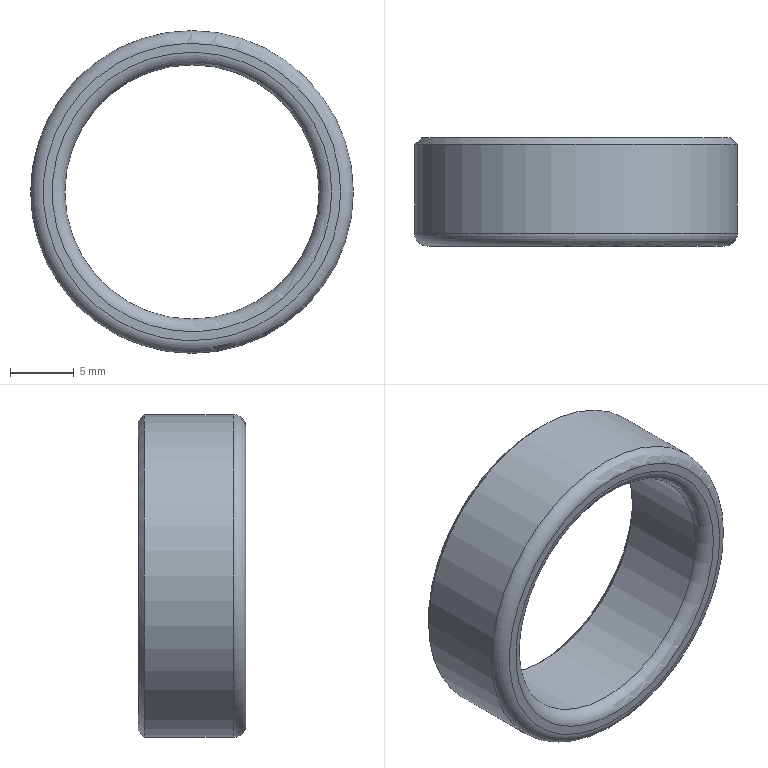Part | STEP file | BK-20_id1170_x_t | 1 solid | 8 faces | box 25.4 x 8.5 x 25.4 mm | volume 1588 mm3 | cylinder 2 | cone 2 | plane 2 | torus 2 | commonest cylinder face diameters 20 x1 25.4 x1
STEP:
#1=CARTESIAN_POINT('',(0.,0.,0.));
#2=DIRECTION('',(0.,0.,1.));
#3=DIRECTION('',(1.,0.,0.));
#4=AXIS2_PLACEMENT_3D('',#1,#2,#3);
#5=CARTESIAN_POINT('',(-258.5,510.436,-165.5));
#6=VERTEX_POINT('',#5);
#7=CARTESIAN_POINT('',(-268.5,510.436,-165.5));
#8=DIRECTION('',(0.,-1.,0.));
#9=DIRECTION('',(1.,0.,0.));
#10=AXIS2_PLACEMENT_3D('',#7,#8,#9);
#11=CIRCLE('',#10,10.);
#12=CARTESIAN_POINT('',(-268.5,494.874,-165.5));
#13=DIRECTION('',(0.,-1.,0.));
#14=DIRECTION('',(1.,0.,0.));
#15=AXIS2_PLACEMENT_3D('',#12,#13,#14);
#16=CYLINDRICAL_SURFACE('',#15,10.);
#17=CARTESIAN_POINT('',(0.,-15.562));
#18=DIRECTION('',(1.,0.));
#19=VECTOR('',#18,1.);
#20=LINE('',#17,#19);
#21=(GEOMETRIC_REPRESENTATION_CONTEXT(2)PARAMETRIC_REPRESENTATION_CONTEXT()REPRESENTATION_CONTEXT('',''));
#22=DEFINITIONAL_REPRESENTATION('',(#20),#21);
#23=PCURVE('',#16,#22);
#24=CARTESIAN_POINT('',(-268.5,510.436,-165.5));
#25=DIRECTION('',(0.,-1.,0.));
#26=DIRECTION('',(1.,0.,0.));
#27=AXIS2_PLACEMENT_3D('',#24,#25,#26);
#28=TOROIDAL_SURFACE('',#27,11.,1.);
#29=CARTESIAN_POINT('',(0.,9.425));
#30=DIRECTION('',(1.,0.));
#31=VECTOR('',#30,1.);
#32=LINE('',#29,#31);
#33=(GEOMETRIC_REPRESENTATION_CONTEXT(2)PARAMETRIC_REPRESENTATION_CONTEXT()REPRESENTATION_CONTEXT('',''));
#34=DEFINITIONAL_REPRESENTATION('',(#32),#33);
#35=PCURVE('',#28,#34);
#36=SURFACE_CURVE('',#11,(#23,#35),.PCURVE_S1.);
#37=EDGE_CURVE('',#6,#6,#36,.T.);
#38=ORIENTED_EDGE('',*,*,#37,.F.);
#39=CARTESIAN_POINT('',(-258.5,517.436,-165.5));
#40=VERTEX_POINT('',#39);
#41=CARTESIAN_POINT('',(-258.5,517.436,-165.5));
#42=CARTESIAN_POINT('',(-258.5,510.436,-165.5));
#43=B_SPLINE_CURVE_WITH_KNOTS('',1,(#41,#42),.UNSPECIFIED.,.F.,.F.,(2,2),(-22.562,-15.562),.PIECEWISE_BEZIER_KNOTS.);
#44=CARTESIAN_POINT('',(0.,0.));
#45=DIRECTION('',(0.,1.));
#46=VECTOR('',#45,1.);
#47=LINE('',#44,#46);
#48=(GEOMETRIC_REPRESENTATION_CONTEXT(2)PARAMETRIC_REPRESENTATION_CONTEXT()REPRESENTATION_CONTEXT('',''));
#49=DEFINITIONAL_REPRESENTATION('',(#47),#48);
#50=PCURVE('',#16,#49);
#51=CARTESIAN_POINT('',(6.283,0.));
#52=DIRECTION('',(0.,1.));
#53=VECTOR('',#52,1.);
#54=LINE('',#51,#53);
#55=(GEOMETRIC_REPRESENTATION_CONTEXT(2)PARAMETRIC_REPRESENTATION_CONTEXT()REPRESENTATION_CONTEXT('',''));
#56=DEFINITIONAL_REPRESENTATION('',(#54),#55);
#57=PCURVE('',#16,#56);
#58=SEAM_CURVE('',#43,(#50,#57),.PCURVE_S1.);
#59=EDGE_CURVE('',#40,#6,#58,.T.);
#60=ORIENTED_EDGE('',*,*,#59,.F.);
#61=CARTESIAN_POINT('',(-278.5,517.436,-165.5));
#62=VERTEX_POINT('',#61);
#63=CARTESIAN_POINT('',(-268.5,517.436,-165.5));
#64=DIRECTION('',(0.,1.,0.));
#65=DIRECTION('',(-1.,0.,0.));
#66=AXIS2_PLACEMENT_3D('',#63,#64,#65);
#67=CIRCLE('',#66,10.);
#68=CARTESIAN_POINT('',(3.142,-22.562));
#69=DIRECTION('',(-1.,0.));
#70=VECTOR('',#69,1.);
#71=LINE('',#68,#70);
#72=(GEOMETRIC_REPRESENTATION_CONTEXT(2)PARAMETRIC_REPRESENTATION_CONTEXT()REPRESENTATION_CONTEXT('',''));
#73=DEFINITIONAL_REPRESENTATION('',(#71),#72);
#74=PCURVE('',#16,#73);
#75=CARTESIAN_POINT('',(-268.5,517.936,-165.5));
#76=DIRECTION('',(0.,1.,0.));
#77=DIRECTION('',(-1.,0.,0.));
#78=AXIS2_PLACEMENT_3D('',#75,#76,#77);
#79=CONICAL_SURFACE('',#78,10.5,0.7854);
#80=CARTESIAN_POINT('',(0.,-0.5));
#81=DIRECTION('',(1.,0.));
#82=VECTOR('',#81,1.);
#83=LINE('',#80,#82);
#84=(GEOMETRIC_REPRESENTATION_CONTEXT(2)PARAMETRIC_REPRESENTATION_CONTEXT()REPRESENTATION_CONTEXT('',''));
#85=DEFINITIONAL_REPRESENTATION('',(#83),#84);
#86=PCURVE('',#79,#85);
#87=SURFACE_CURVE('',#67,(#74,#86),.PCURVE_S1.);
#88=EDGE_CURVE('',#62,#40,#87,.T.);
#89=ORIENTED_EDGE('',*,*,#88,.F.);
#90=CARTESIAN_POINT('',(-268.5,517.436,-165.5));
#91=DIRECTION('',(0.,1.,0.));
#92=DIRECTION('',(-1.,0.,0.));
#93=AXIS2_PLACEMENT_3D('',#90,#91,#92);
#94=CIRCLE('',#93,10.);
#95=CARTESIAN_POINT('',(9.425,-22.562));
#96=DIRECTION('',(-1.,0.));
#97=VECTOR('',#96,1.);
#98=LINE('',#95,#97);
#99=(GEOMETRIC_REPRESENTATION_CONTEXT(2)PARAMETRIC_REPRESENTATION_CONTEXT()REPRESENTATION_CONTEXT('',''));
#100=DEFINITIONAL_REPRESENTATION('',(#98),#99);
#101=PCURVE('',#16,#100);
#102=CARTESIAN_POINT('',(0.,-0.5));
#103=DIRECTION('',(1.,0.));
#104=VECTOR('',#103,1.);
#105=LINE('',#102,#104);
#106=(GEOMETRIC_REPRESENTATION_CONTEXT(2)PARAMETRIC_REPRESENTATION_CONTEXT()REPRESENTATION_CONTEXT('',''));
#107=DEFINITIONAL_REPRESENTATION('',(#105),#106);
#108=PCURVE('',#79,#107);
#109=SURFACE_CURVE('',#94,(#101,#108),.PCURVE_S1.);
#110=EDGE_CURVE('',#40,#62,#109,.T.);
#111=ORIENTED_EDGE('',*,*,#110,.F.);
#112=ORIENTED_EDGE('',*,*,#59,.T.);
#113=EDGE_LOOP('',(#38,#60,#89,#111,#112));
#114=FACE_BOUND('',#113,.F.);
#115=ADVANCED_FACE('',(#114),#16,.F.);
#116=ORIENTED_EDGE('',*,*,#110,.T.);
#117=CARTESIAN_POINT('',(-279.,517.936,-165.5));
#118=VERTEX_POINT('',#117);
#119=CARTESIAN_POINT('',(-278.5,517.436,-165.5));
#120=CARTESIAN_POINT('',(-279.,517.936,-165.5));
#121=B_SPLINE_CURVE_WITH_KNOTS('',1,(#119,#120),.UNSPECIFIED.,.F.,.F.,(2,2),(-0.7071,0.),.PIECEWISE_BEZIER_KNOTS.);
#122=CARTESIAN_POINT('',(6.283,0.));
#123=DIRECTION('',(0.,1.));
#124=VECTOR('',#123,1.);
#125=LINE('',#122,#124);
#126=(GEOMETRIC_REPRESENTATION_CONTEXT(2)PARAMETRIC_REPRESENTATION_CONTEXT()REPRESENTATION_CONTEXT('',''));
#127=DEFINITIONAL_REPRESENTATION('',(#125),#126);
#128=PCURVE('',#79,#127);
#129=CARTESIAN_POINT('',(0.,0.));
#130=DIRECTION('',(0.,1.));
#131=VECTOR('',#130,1.);
#132=LINE('',#129,#131);
#133=(GEOMETRIC_REPRESENTATION_CONTEXT(2)PARAMETRIC_REPRESENTATION_CONTEXT()REPRESENTATION_CONTEXT('',''));
#134=DEFINITIONAL_REPRESENTATION('',(#132),#133);
#135=PCURVE('',#79,#134);
#136=SEAM_CURVE('',#121,(#128,#135),.PCURVE_S1.);
#137=EDGE_CURVE('',#62,#118,#136,.T.);
#138=ORIENTED_EDGE('',*,*,#137,.T.);
#139=CARTESIAN_POINT('',(-268.5,517.936,-165.5));
#140=DIRECTION('',(0.,1.,0.));
#141=DIRECTION('',(-1.,0.,0.));
#142=AXIS2_PLACEMENT_3D('',#139,#140,#141);
#143=CIRCLE('',#142,10.5);
#144=CARTESIAN_POINT('',(0.,0.));
#145=DIRECTION('',(1.,0.));
#146=VECTOR('',#145,1.);
#147=LINE('',#144,#146);
#148=(GEOMETRIC_REPRESENTATION_CONTEXT(2)PARAMETRIC_REPRESENTATION_CONTEXT()REPRESENTATION_CONTEXT('',''));
#149=DEFINITIONAL_REPRESENTATION('',(#147),#148);
#150=PCURVE('',#79,#149);
#151=CARTESIAN_POINT('',(-268.5,517.936,-152.8));
#152=DIRECTION('',(0.,-1.,0.));
#153=DIRECTION('',(1.,0.,0.));
#154=AXIS2_PLACEMENT_3D('',#151,#152,#153);
#155=PLANE('',#154);
#156=CARTESIAN_POINT('',(-10.5,-12.7));
#157=CARTESIAN_POINT('',(-10.5,5.487));
#158=CARTESIAN_POINT('',(5.25,-3.607));
#159=CARTESIAN_POINT('',(21.,-12.7));
#160=CARTESIAN_POINT('',(5.25,-21.793));
#161=CARTESIAN_POINT('',(-10.5,-30.887));
#162=CARTESIAN_POINT('',(-10.5,-12.7));
#163=(BOUNDED_CURVE()B_SPLINE_CURVE(2,(#156,#157,#158,#159,#160,#161,#162),.UNSPECIFIED.,.T.,.F.)B_SPLINE_CURVE_WITH_KNOTS((1,2,2,2,2,1),(-2.094,0.,2.094,4.189,6.283,8.378),.UNSPECIFIED.)CURVE()GEOMETRIC_REPRESENTATION_ITEM()RATIONAL_B_SPLINE_CURVE((1.,0.5,1.,0.5,1.,0.5,1.))REPRESENTATION_ITEM(''));
#164=(GEOMETRIC_REPRESENTATION_CONTEXT(2)PARAMETRIC_REPRESENTATION_CONTEXT()REPRESENTATION_CONTEXT('',''));
#165=DEFINITIONAL_REPRESENTATION('',(#163),#164);
#166=PCURVE('',#155,#165);
#167=SURFACE_CURVE('',#143,(#150,#166),.PCURVE_S1.);
#168=EDGE_CURVE('',#118,#118,#167,.T.);
#169=ORIENTED_EDGE('',*,*,#168,.F.);
#170=ORIENTED_EDGE('',*,*,#137,.F.);
#171=ORIENTED_EDGE('',*,*,#88,.T.);
#172=EDGE_LOOP('',(#116,#138,#169,#170,#171));
#173=FACE_BOUND('',#172,.F.);
#174=ADVANCED_FACE('',(#173),#79,.F.);
#175=ORIENTED_EDGE('',*,*,#168,.F.);
#176=EDGE_LOOP('',(#175));
#177=FACE_BOUND('',#176,.T.);
#178=CARTESIAN_POINT('',(-256.3,517.936,-165.5));
#179=VERTEX_POINT('',#178);
#180=CARTESIAN_POINT('',(-268.5,517.936,-165.5));
#181=DIRECTION('',(0.,-1.,0.));
#182=DIRECTION('',(1.,0.,0.));
#183=AXIS2_PLACEMENT_3D('',#180,#181,#182);
#184=CIRCLE('',#183,12.2);
#185=CARTESIAN_POINT('',(0.,-12.7));
#186=DIRECTION('',(1.,0.));
#187=AXIS2_PLACEMENT_2D('',#185,#186);
#188=CIRCLE('',#187,12.2);
#189=(GEOMETRIC_REPRESENTATION_CONTEXT(2)PARAMETRIC_REPRESENTATION_CONTEXT()REPRESENTATION_CONTEXT('',''));
#190=DEFINITIONAL_REPRESENTATION('',(#188),#189);
#191=PCURVE('',#155,#190);
#192=CARTESIAN_POINT('',(-268.5,517.436,-165.5));
#193=DIRECTION('',(0.,-1.,0.));
#194=DIRECTION('',(1.,0.,0.));
#195=AXIS2_PLACEMENT_3D('',#192,#193,#194);
#196=CONICAL_SURFACE('',#195,12.7,0.7854);
#197=CARTESIAN_POINT('',(0.,-0.5));
#198=DIRECTION('',(1.,0.));
#199=VECTOR('',#198,1.);
#200=LINE('',#197,#199);
#201=(GEOMETRIC_REPRESENTATION_CONTEXT(2)PARAMETRIC_REPRESENTATION_CONTEXT()REPRESENTATION_CONTEXT('',''));
#202=DEFINITIONAL_REPRESENTATION('',(#200),#201);
#203=PCURVE('',#196,#202);
#204=SURFACE_CURVE('',#184,(#191,#203),.PCURVE_S1.);
#205=EDGE_CURVE('',#179,#179,#204,.T.);
#206=ORIENTED_EDGE('',*,*,#205,.F.);
#207=EDGE_LOOP('',(#206));
#208=FACE_BOUND('',#207,.T.);
#209=ADVANCED_FACE('',(#177,#208),#155,.F.);
#210=CARTESIAN_POINT('',(-255.8,517.436,-165.5));
#211=VERTEX_POINT('',#210);
#212=CARTESIAN_POINT('',(-268.5,517.436,-165.5));
#213=DIRECTION('',(0.,-1.,0.));
#214=DIRECTION('',(1.,0.,0.));
#215=AXIS2_PLACEMENT_3D('',#212,#213,#214);
#216=CIRCLE('',#215,12.7);
#217=CARTESIAN_POINT('',(0.,0.));
#218=DIRECTION('',(1.,0.));
#219=VECTOR('',#218,1.);
#220=LINE('',#217,#219);
#221=(GEOMETRIC_REPRESENTATION_CONTEXT(2)PARAMETRIC_REPRESENTATION_CONTEXT()REPRESENTATION_CONTEXT('',''));
#222=DEFINITIONAL_REPRESENTATION('',(#220),#221);
#223=PCURVE('',#196,#222);
#224=CARTESIAN_POINT('',(-268.5,494.874,-165.5));
#225=DIRECTION('',(0.,-1.,0.));
#226=DIRECTION('',(1.,0.,0.));
#227=AXIS2_PLACEMENT_3D('',#224,#225,#226);
#228=CYLINDRICAL_SURFACE('',#227,12.7);
#229=CARTESIAN_POINT('',(0.,-22.562));
#230=DIRECTION('',(1.,0.));
#231=VECTOR('',#230,1.);
#232=LINE('',#229,#231);
#233=(GEOMETRIC_REPRESENTATION_CONTEXT(2)PARAMETRIC_REPRESENTATION_CONTEXT()REPRESENTATION_CONTEXT('',''));
#234=DEFINITIONAL_REPRESENTATION('',(#232),#233);
#235=PCURVE('',#228,#234);
#236=SURFACE_CURVE('',#216,(#223,#235),.PCURVE_S1.);
#237=EDGE_CURVE('',#211,#211,#236,.T.);
#238=ORIENTED_EDGE('',*,*,#237,.F.);
#239=CARTESIAN_POINT('',(-256.3,517.936,-165.5));
#240=CARTESIAN_POINT('',(-255.8,517.436,-165.5));
#241=B_SPLINE_CURVE_WITH_KNOTS('',1,(#239,#240),.UNSPECIFIED.,.F.,.F.,(2,2),(-0.7071,0.),.PIECEWISE_BEZIER_KNOTS.);
#242=CARTESIAN_POINT('',(0.,0.));
#243=DIRECTION('',(0.,1.));
#244=VECTOR('',#243,1.);
#245=LINE('',#242,#244);
#246=(GEOMETRIC_REPRESENTATION_CONTEXT(2)PARAMETRIC_REPRESENTATION_CONTEXT()REPRESENTATION_CONTEXT('',''));
#247=DEFINITIONAL_REPRESENTATION('',(#245),#246);
#248=PCURVE('',#196,#247);
#249=CARTESIAN_POINT('',(6.283,0.));
#250=DIRECTION('',(0.,1.));
#251=VECTOR('',#250,1.);
#252=LINE('',#249,#251);
#253=(GEOMETRIC_REPRESENTATION_CONTEXT(2)PARAMETRIC_REPRESENTATION_CONTEXT()REPRESENTATION_CONTEXT('',''));
#254=DEFINITIONAL_REPRESENTATION('',(#252),#253);
#255=PCURVE('',#196,#254);
#256=SEAM_CURVE('',#241,(#248,#255),.PCURVE_S1.);
#257=EDGE_CURVE('',#179,#211,#256,.T.);
#258=ORIENTED_EDGE('',*,*,#257,.F.);
#259=ORIENTED_EDGE('',*,*,#205,.T.);
#260=ORIENTED_EDGE('',*,*,#257,.T.);
#261=EDGE_LOOP('',(#238,#258,#259,#260));
#262=FACE_BOUND('',#261,.T.);
#263=ADVANCED_FACE('',(#262),#196,.T.);
#264=CARTESIAN_POINT('',(-255.8,510.436,-165.5));
#265=VERTEX_POINT('',#264);
#266=CARTESIAN_POINT('',(-268.5,510.436,-165.5));
#267=DIRECTION('',(0.,1.,0.));
#268=DIRECTION('',(1.,0.,0.));
#269=AXIS2_PLACEMENT_3D('',#266,#267,#268);
#270=CIRCLE('',#269,12.7);
#271=CARTESIAN_POINT('',(6.283,-15.562));
#272=DIRECTION('',(-1.,0.));
#273=VECTOR('',#272,1.);
#274=LINE('',#271,#273);
#275=(GEOMETRIC_REPRESENTATION_CONTEXT(2)PARAMETRIC_REPRESENTATION_CONTEXT()REPRESENTATION_CONTEXT('',''));
#276=DEFINITIONAL_REPRESENTATION('',(#274),#275);
#277=PCURVE('',#228,#276);
#278=CARTESIAN_POINT('',(-268.5,510.436,-165.5));
#279=DIRECTION('',(0.,-1.,0.));
#280=DIRECTION('',(1.,0.,0.));
#281=AXIS2_PLACEMENT_3D('',#278,#279,#280);
#282=TOROIDAL_SURFACE('',#281,11.7,1.);
#283=CARTESIAN_POINT('',(6.283,6.283));
#284=DIRECTION('',(-1.,0.));
#285=VECTOR('',#284,1.);
#286=LINE('',#283,#285);
#287=(GEOMETRIC_REPRESENTATION_CONTEXT(2)PARAMETRIC_REPRESENTATION_CONTEXT()REPRESENTATION_CONTEXT('',''));
#288=DEFINITIONAL_REPRESENTATION('',(#286),#287);
#289=PCURVE('',#282,#288);
#290=SURFACE_CURVE('',#270,(#277,#289),.PCURVE_S1.);
#291=EDGE_CURVE('',#265,#265,#290,.T.);
#292=ORIENTED_EDGE('',*,*,#291,.T.);
#293=CARTESIAN_POINT('',(-255.8,517.436,-165.5));
#294=CARTESIAN_POINT('',(-255.8,510.436,-165.5));
#295=B_SPLINE_CURVE_WITH_KNOTS('',1,(#293,#294),.UNSPECIFIED.,.F.,.F.,(2,2),(-22.562,-15.562),.PIECEWISE_BEZIER_KNOTS.);
#296=CARTESIAN_POINT('',(0.,0.));
#297=DIRECTION('',(0.,1.));
#298=VECTOR('',#297,1.);
#299=LINE('',#296,#298);
#300=(GEOMETRIC_REPRESENTATION_CONTEXT(2)PARAMETRIC_REPRESENTATION_CONTEXT()REPRESENTATION_CONTEXT('',''));
#301=DEFINITIONAL_REPRESENTATION('',(#299),#300);
#302=PCURVE('',#228,#301);
#303=CARTESIAN_POINT('',(6.283,0.));
#304=DIRECTION('',(0.,1.));
#305=VECTOR('',#304,1.);
#306=LINE('',#303,#305);
#307=(GEOMETRIC_REPRESENTATION_CONTEXT(2)PARAMETRIC_REPRESENTATION_CONTEXT()REPRESENTATION_CONTEXT('',''));
#308=DEFINITIONAL_REPRESENTATION('',(#306),#307);
#309=PCURVE('',#228,#308);
#310=SEAM_CURVE('',#295,(#302,#309),.PCURVE_S1.);
#311=EDGE_CURVE('',#211,#265,#310,.T.);
#312=ORIENTED_EDGE('',*,*,#311,.F.);
#313=ORIENTED_EDGE('',*,*,#237,.T.);
#314=ORIENTED_EDGE('',*,*,#311,.T.);
#315=EDGE_LOOP('',(#292,#312,#313,#314));
#316=FACE_BOUND('',#315,.T.);
#317=ADVANCED_FACE('',(#316),#228,.T.);
#318=CARTESIAN_POINT('',(-257.5,509.436,-165.5));
#319=VERTEX_POINT('',#318);
#320=CARTESIAN_POINT('',(-268.5,509.436,-165.5));
#321=DIRECTION('',(0.,1.,0.));
#322=DIRECTION('',(1.,0.,0.));
#323=AXIS2_PLACEMENT_3D('',#320,#321,#322);
#324=CIRCLE('',#323,11.);
#325=CARTESIAN_POINT('',(-268.5,509.436,-165.5));
#326=DIRECTION('',(0.,-1.,0.));
#327=DIRECTION('',(1.,0.,0.));
#328=AXIS2_PLACEMENT_3D('',#325,#326,#327);
#329=PLANE('',#328);
#330=CARTESIAN_POINT('',(11.,0.));
#331=CARTESIAN_POINT('',(11.,-19.053));
#332=CARTESIAN_POINT('',(-5.5,-9.526));
#333=CARTESIAN_POINT('',(-22.,0.));
#334=CARTESIAN_POINT('',(-5.5,9.526));
#335=CARTESIAN_POINT('',(11.,19.053));
#336=CARTESIAN_POINT('',(11.,0.));
#337=(BOUNDED_CURVE()B_SPLINE_CURVE(2,(#330,#331,#332,#333,#334,#335,#336),.UNSPECIFIED.,.T.,.F.)B_SPLINE_CURVE_WITH_KNOTS((1,2,2,2,2,1),(-2.094,0.,2.094,4.189,6.283,8.378),.UNSPECIFIED.)CURVE()GEOMETRIC_REPRESENTATION_ITEM()RATIONAL_B_SPLINE_CURVE((1.,0.5,1.,0.5,1.,0.5,1.))REPRESENTATION_ITEM(''));
#338=(GEOMETRIC_REPRESENTATION_CONTEXT(2)PARAMETRIC_REPRESENTATION_CONTEXT()REPRESENTATION_CONTEXT('',''));
#339=DEFINITIONAL_REPRESENTATION('',(#337),#338);
#340=PCURVE('',#329,#339);
#341=CARTESIAN_POINT('',(6.283,7.854));
#342=DIRECTION('',(-1.,0.));
#343=VECTOR('',#342,1.);
#344=LINE('',#341,#343);
#345=(GEOMETRIC_REPRESENTATION_CONTEXT(2)PARAMETRIC_REPRESENTATION_CONTEXT()REPRESENTATION_CONTEXT('',''));
#346=DEFINITIONAL_REPRESENTATION('',(#344),#345);
#347=PCURVE('',#28,#346);
#348=SURFACE_CURVE('',#324,(#340,#347),.PCURVE_S1.);
#349=EDGE_CURVE('',#319,#319,#348,.T.);
#350=ORIENTED_EDGE('',*,*,#349,.T.);
#351=EDGE_LOOP('',(#350));
#352=FACE_BOUND('',#351,.T.);
#353=CARTESIAN_POINT('',(-256.8,509.436,-165.5));
#354=VERTEX_POINT('',#353);
#355=CARTESIAN_POINT('',(-268.5,509.436,-165.5));
#356=DIRECTION('',(0.,-1.,0.));
#357=DIRECTION('',(1.,0.,0.));
#358=AXIS2_PLACEMENT_3D('',#355,#356,#357);
#359=CIRCLE('',#358,11.7);
#360=CARTESIAN_POINT('',(0.,0.));
#361=DIRECTION('',(1.,0.));
#362=AXIS2_PLACEMENT_2D('',#360,#361);
#363=CIRCLE('',#362,11.7);
#364=(GEOMETRIC_REPRESENTATION_CONTEXT(2)PARAMETRIC_REPRESENTATION_CONTEXT()REPRESENTATION_CONTEXT('',''));
#365=DEFINITIONAL_REPRESENTATION('',(#363),#364);
#366=PCURVE('',#329,#365);
#367=CARTESIAN_POINT('',(0.,7.854));
#368=DIRECTION('',(1.,0.));
#369=VECTOR('',#368,1.);
#370=LINE('',#367,#369);
#371=(GEOMETRIC_REPRESENTATION_CONTEXT(2)PARAMETRIC_REPRESENTATION_CONTEXT()REPRESENTATION_CONTEXT('',''));
#372=DEFINITIONAL_REPRESENTATION('',(#370),#371);
#373=PCURVE('',#282,#372);
#374=SURFACE_CURVE('',#359,(#366,#373),.PCURVE_S1.);
#375=EDGE_CURVE('',#354,#354,#374,.T.);
#376=ORIENTED_EDGE('',*,*,#375,.T.);
#377=EDGE_LOOP('',(#376));
#378=FACE_BOUND('',#377,.T.);
#379=ADVANCED_FACE('',(#352,#378),#329,.T.);
#380=ORIENTED_EDGE('',*,*,#349,.F.);
#381=CARTESIAN_POINT('',(-257.5,509.436,-165.5));
#382=CARTESIAN_POINT('',(-257.767,509.436,-165.5));
#383=CARTESIAN_POINT('',(-258.028,509.521,-165.5));
#384=CARTESIAN_POINT('',(-258.252,509.684,-165.5));
#385=CARTESIAN_POINT('',(-258.415,509.908,-165.5));
#386=CARTESIAN_POINT('',(-258.5,510.168,-165.5));
#387=CARTESIAN_POINT('',(-258.5,510.436,-165.5));
#388=(BOUNDED_CURVE()B_SPLINE_CURVE(6,(#381,#382,#383,#384,#385,#386,#387),.UNSPECIFIED.,.F.,.F.)B_SPLINE_CURVE_WITH_KNOTS((7,7),(1.571,3.142),.PIECEWISE_BEZIER_KNOTS.)CURVE()GEOMETRIC_REPRESENTATION_ITEM()RATIONAL_B_SPLINE_CURVE((1.031,1.01,0.9979,0.994,0.9979,1.01,1.031))REPRESENTATION_ITEM(''));
#389=CARTESIAN_POINT('',(6.283,6.283));
#390=DIRECTION('',(0.,1.));
#391=VECTOR('',#390,1.);
#392=LINE('',#389,#391);
#393=(GEOMETRIC_REPRESENTATION_CONTEXT(2)PARAMETRIC_REPRESENTATION_CONTEXT()REPRESENTATION_CONTEXT('',''));
#394=DEFINITIONAL_REPRESENTATION('',(#392),#393);
#395=PCURVE('',#28,#394);
#396=CARTESIAN_POINT('',(0.,6.283));
#397=DIRECTION('',(0.,1.));
#398=VECTOR('',#397,1.);
#399=LINE('',#396,#398);
#400=(GEOMETRIC_REPRESENTATION_CONTEXT(2)PARAMETRIC_REPRESENTATION_CONTEXT()REPRESENTATION_CONTEXT('',''));
#401=DEFINITIONAL_REPRESENTATION('',(#399),#400);
#402=PCURVE('',#28,#401);
#403=SEAM_CURVE('',#388,(#395,#402),.PCURVE_S1.);
#404=EDGE_CURVE('',#319,#6,#403,.T.);
#405=ORIENTED_EDGE('',*,*,#404,.T.);
#406=ORIENTED_EDGE('',*,*,#37,.F.);
#407=ORIENTED_EDGE('',*,*,#404,.F.);
#408=EDGE_LOOP('',(#380,#405,#406,#407));
#409=FACE_BOUND('',#408,.T.);
#410=ADVANCED_FACE('',(#409),#28,.T.);
#411=ORIENTED_EDGE('',*,*,#291,.F.);
#412=CARTESIAN_POINT('',(-255.8,510.436,-165.5));
#413=CARTESIAN_POINT('',(-255.8,510.168,-165.5));
#414=CARTESIAN_POINT('',(-255.885,509.908,-165.5));
#415=CARTESIAN_POINT('',(-256.048,509.684,-165.5));
#416=CARTESIAN_POINT('',(-256.272,509.521,-165.5));
#417=CARTESIAN_POINT('',(-256.533,509.436,-165.5));
#418=CARTESIAN_POINT('',(-256.8,509.436,-165.5));
#419=(BOUNDED_CURVE()B_SPLINE_CURVE(6,(#412,#413,#414,#415,#416,#417,#418),.UNSPECIFIED.,.F.,.F.)B_SPLINE_CURVE_WITH_KNOTS((7,7),(0.,1.571),.PIECEWISE_BEZIER_KNOTS.)CURVE()GEOMETRIC_REPRESENTATION_ITEM()RATIONAL_B_SPLINE_CURVE((1.031,1.01,0.9979,0.994,0.9979,1.01,1.031))REPRESENTATION_ITEM(''));
#420=CARTESIAN_POINT('',(6.283,6.283));
#421=DIRECTION('',(0.,1.));
#422=VECTOR('',#421,1.);
#423=LINE('',#420,#422);
#424=(GEOMETRIC_REPRESENTATION_CONTEXT(2)PARAMETRIC_REPRESENTATION_CONTEXT()REPRESENTATION_CONTEXT('',''));
#425=DEFINITIONAL_REPRESENTATION('',(#423),#424);
#426=PCURVE('',#282,#425);
#427=CARTESIAN_POINT('',(0.,6.283));
#428=DIRECTION('',(0.,1.));
#429=VECTOR('',#428,1.);
#430=LINE('',#427,#429);
#431=(GEOMETRIC_REPRESENTATION_CONTEXT(2)PARAMETRIC_REPRESENTATION_CONTEXT()REPRESENTATION_CONTEXT('',''));
#432=DEFINITIONAL_REPRESENTATION('',(#430),#431);
#433=PCURVE('',#282,#432);
#434=SEAM_CURVE('',#419,(#426,#433),.PCURVE_S1.);
#435=EDGE_CURVE('',#265,#354,#434,.T.);
#436=ORIENTED_EDGE('',*,*,#435,.T.);
#437=ORIENTED_EDGE('',*,*,#375,.F.);
#438=ORIENTED_EDGE('',*,*,#435,.F.);
#439=EDGE_LOOP('',(#411,#436,#437,#438));
#440=FACE_BOUND('',#439,.T.);
#441=ADVANCED_FACE('',(#440),#282,.T.);
#442=CLOSED_SHELL('',(#115,#174,#209,#263,#317,#379,#410,#441));
#443=MANIFOLD_SOLID_BREP('',#442);
#444=(LENGTH_UNIT()NAMED_UNIT(*)SI_UNIT(.MILLI.,.METRE.));
#445=UNCERTAINTY_MEASURE_WITH_UNIT(LENGTH_MEASURE(0.00001),#444,'','');
#446=(NAMED_UNIT(*)PLANE_ANGLE_UNIT()SI_UNIT($,.RADIAN.));
#447=(NAMED_UNIT(*)SI_UNIT($,.STERADIAN.)SOLID_ANGLE_UNIT());
#448=(GEOMETRIC_REPRESENTATION_CONTEXT(3)GLOBAL_UNCERTAINTY_ASSIGNED_CONTEXT((#445))GLOBAL_UNIT_ASSIGNED_CONTEXT((#444,#446,#447))REPRESENTATION_CONTEXT('',''));
#449=ADVANCED_BREP_SHAPE_REPRESENTATION('',(#4,#443),#448);